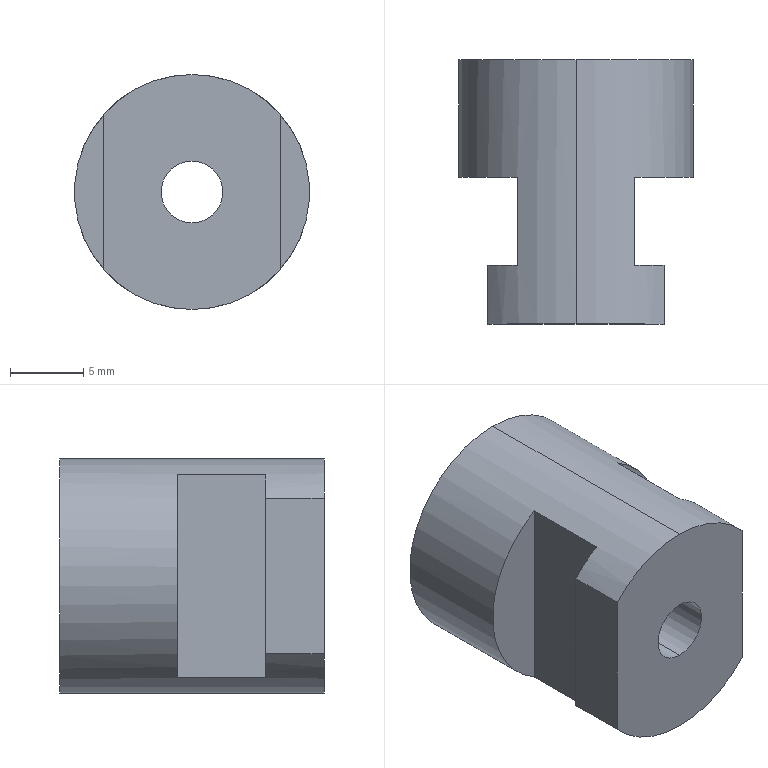Part | STEP file | 16 union cap | 1 solid | 14 faces | box 16 x 18 x 16 mm | volume 2782 mm3 | plane 10 | cylinder 4 | commonest cylinder face diameters 4.2 x2 16 x2
STEP:
#1=CARTESIAN_POINT('',(0.,0.,0.));
#2=DIRECTION('',(0.,0.,1.));
#3=DIRECTION('',(1.,0.,0.));
#4=AXIS2_PLACEMENT_3D('',#1,#2,#3);
#5=CARTESIAN_POINT('',(3.464,10.483,-2.1));
#6=VERTEX_POINT('',#5);
#7=CARTESIAN_POINT('',(3.464,-7.517,-2.1));
#8=VERTEX_POINT('',#7);
#9=CARTESIAN_POINT('',(3.464,-7.517,-2.1));
#10=DIRECTION('',(0.,-1.,0.));
#11=VECTOR('',#10,1.);
#12=LINE('',#9,#11);
#13=CARTESIAN_POINT('',(3.464,-7.517,0.));
#14=DIRECTION('',(0.,-1.,0.));
#15=DIRECTION('',(0.,0.,-1.));
#16=AXIS2_PLACEMENT_3D('',#13,#14,#15);
#17=CYLINDRICAL_SURFACE('',#16,2.1);
#18=CARTESIAN_POINT('',(6.283,0.));
#19=DIRECTION('',(0.,1.));
#20=VECTOR('',#19,1.);
#21=LINE('',#18,#20);
#22=(GEOMETRIC_REPRESENTATION_CONTEXT(2)PARAMETRIC_REPRESENTATION_CONTEXT()REPRESENTATION_CONTEXT('',''));
#23=DEFINITIONAL_REPRESENTATION('',(#21),#22);
#24=PCURVE('',#17,#23);
#25=CARTESIAN_POINT('',(3.464,-7.517,0.));
#26=DIRECTION('',(0.,-1.,0.));
#27=DIRECTION('',(0.,0.,-1.));
#28=AXIS2_PLACEMENT_3D('',#25,#26,#27);
#29=CYLINDRICAL_SURFACE('',#28,2.1);
#30=CARTESIAN_POINT('',(0.,0.));
#31=DIRECTION('',(0.,1.));
#32=VECTOR('',#31,1.);
#33=LINE('',#30,#32);
#34=(GEOMETRIC_REPRESENTATION_CONTEXT(2)PARAMETRIC_REPRESENTATION_CONTEXT()REPRESENTATION_CONTEXT('',''));
#35=DEFINITIONAL_REPRESENTATION('',(#33),#34);
#36=PCURVE('',#29,#35);
#37=SURFACE_CURVE('',#12,(#24,#36),.PCURVE_S1.);
#38=EDGE_CURVE('',#6,#8,#37,.T.);
#39=ORIENTED_EDGE('',*,*,#38,.T.);
#40=CARTESIAN_POINT('',(3.464,-7.517,2.1));
#41=VERTEX_POINT('',#40);
#42=CARTESIAN_POINT('',(3.464,-7.517,0.));
#43=DIRECTION('',(0.,-1.,0.));
#44=DIRECTION('',(0.,0.,-1.));
#45=AXIS2_PLACEMENT_3D('',#42,#43,#44);
#46=CIRCLE('',#45,2.1);
#47=CARTESIAN_POINT('',(0.,0.));
#48=DIRECTION('',(1.,0.));
#49=VECTOR('',#48,1.);
#50=LINE('',#47,#49);
#51=(GEOMETRIC_REPRESENTATION_CONTEXT(2)PARAMETRIC_REPRESENTATION_CONTEXT()REPRESENTATION_CONTEXT('',''));
#52=DEFINITIONAL_REPRESENTATION('',(#50),#51);
#53=PCURVE('',#17,#52);
#54=CARTESIAN_POINT('',(9.464,-7.517,-10.));
#55=DIRECTION('',(0.,-1.,0.));
#56=DIRECTION('',(0.,0.,-1.));
#57=AXIS2_PLACEMENT_3D('',#54,#55,#56);
#58=PLANE('',#57);
#59=CARTESIAN_POINT('',(-10.,-6.));
#60=DIRECTION('',(1.,0.));
#61=AXIS2_PLACEMENT_2D('',#59,#60);
#62=CIRCLE('',#61,2.1);
#63=(GEOMETRIC_REPRESENTATION_CONTEXT(2)PARAMETRIC_REPRESENTATION_CONTEXT()REPRESENTATION_CONTEXT('',''));
#64=DEFINITIONAL_REPRESENTATION('',(#62),#63);
#65=PCURVE('',#58,#64);
#66=SURFACE_CURVE('',#46,(#53,#65),.PCURVE_S1.);
#67=EDGE_CURVE('',#41,#8,#66,.T.);
#68=ORIENTED_EDGE('',*,*,#67,.F.);
#69=CARTESIAN_POINT('',(3.464,10.483,2.1));
#70=VERTEX_POINT('',#69);
#71=CARTESIAN_POINT('',(3.464,-7.517,2.1));
#72=DIRECTION('',(0.,-1.,0.));
#73=VECTOR('',#72,1.);
#74=LINE('',#71,#73);
#75=CARTESIAN_POINT('',(3.142,0.));
#76=DIRECTION('',(0.,1.));
#77=VECTOR('',#76,1.);
#78=LINE('',#75,#77);
#79=(GEOMETRIC_REPRESENTATION_CONTEXT(2)PARAMETRIC_REPRESENTATION_CONTEXT()REPRESENTATION_CONTEXT('',''));
#80=DEFINITIONAL_REPRESENTATION('',(#78),#79);
#81=PCURVE('',#17,#80);
#82=CARTESIAN_POINT('',(3.142,0.));
#83=DIRECTION('',(0.,1.));
#84=VECTOR('',#83,1.);
#85=LINE('',#82,#84);
#86=(GEOMETRIC_REPRESENTATION_CONTEXT(2)PARAMETRIC_REPRESENTATION_CONTEXT()REPRESENTATION_CONTEXT('',''));
#87=DEFINITIONAL_REPRESENTATION('',(#85),#86);
#88=PCURVE('',#29,#87);
#89=SURFACE_CURVE('',#74,(#81,#88),.PCURVE_S1.);
#90=EDGE_CURVE('',#70,#41,#89,.T.);
#91=ORIENTED_EDGE('',*,*,#90,.F.);
#92=CARTESIAN_POINT('',(3.464,10.483,0.));
#93=DIRECTION('',(0.,-1.,0.));
#94=DIRECTION('',(0.,0.,-1.));
#95=AXIS2_PLACEMENT_3D('',#92,#93,#94);
#96=CIRCLE('',#95,2.1);
#97=CARTESIAN_POINT('',(0.,-18.));
#98=DIRECTION('',(1.,0.));
#99=VECTOR('',#98,1.);
#100=LINE('',#97,#99);
#101=(GEOMETRIC_REPRESENTATION_CONTEXT(2)PARAMETRIC_REPRESENTATION_CONTEXT()REPRESENTATION_CONTEXT('',''));
#102=DEFINITIONAL_REPRESENTATION('',(#100),#101);
#103=PCURVE('',#17,#102);
#104=CARTESIAN_POINT('',(3.464,10.483,0.));
#105=DIRECTION('',(0.,1.,0.));
#106=DIRECTION('',(0.,0.,1.));
#107=AXIS2_PLACEMENT_3D('',#104,#105,#106);
#108=PLANE('',#107);
#109=CARTESIAN_POINT('',(-2.1,0.));
#110=CARTESIAN_POINT('',(-2.1,3.637));
#111=CARTESIAN_POINT('',(1.05,1.819));
#112=CARTESIAN_POINT('',(4.2,0.));
#113=CARTESIAN_POINT('',(1.05,-1.819));
#114=CARTESIAN_POINT('',(-2.1,-3.637));
#115=CARTESIAN_POINT('',(-2.1,0.));
#116=(BOUNDED_CURVE()B_SPLINE_CURVE(2,(#109,#110,#111,#112,#113,#114,#115),.UNSPECIFIED.,.T.,.F.)B_SPLINE_CURVE_WITH_KNOTS((1,2,2,2,2,1),(-2.094,0.,2.094,4.189,6.283,8.378),.UNSPECIFIED.)CURVE()GEOMETRIC_REPRESENTATION_ITEM()RATIONAL_B_SPLINE_CURVE((1.,0.5,1.,0.5,1.,0.5,1.))REPRESENTATION_ITEM(''));
#117=(GEOMETRIC_REPRESENTATION_CONTEXT(2)PARAMETRIC_REPRESENTATION_CONTEXT()REPRESENTATION_CONTEXT('',''));
#118=DEFINITIONAL_REPRESENTATION('',(#116),#117);
#119=PCURVE('',#108,#118);
#120=SURFACE_CURVE('',#96,(#103,#119),.PCURVE_S1.);
#121=EDGE_CURVE('',#70,#6,#120,.T.);
#122=ORIENTED_EDGE('',*,*,#121,.T.);
#123=EDGE_LOOP('',(#39,#68,#91,#122));
#124=FACE_BOUND('',#123,.F.);
#125=ADVANCED_FACE('',(#124),#17,.F.);
#126=CARTESIAN_POINT('',(9.464,-7.517,-5.292));
#127=VERTEX_POINT('',#126);
#128=CARTESIAN_POINT('',(3.464,-7.517,-8.));
#129=VERTEX_POINT('',#128);
#130=CARTESIAN_POINT('',(3.464,-7.517,0.));
#131=DIRECTION('',(0.,1.,0.));
#132=DIRECTION('',(0.,0.,1.));
#133=AXIS2_PLACEMENT_3D('',#130,#131,#132);
#134=CIRCLE('',#133,8.);
#135=CARTESIAN_POINT('',(3.464,-7.517,0.));
#136=DIRECTION('',(0.,1.,0.));
#137=DIRECTION('',(0.,0.,1.));
#138=AXIS2_PLACEMENT_3D('',#135,#136,#137);
#139=CYLINDRICAL_SURFACE('',#138,8.);
#140=CARTESIAN_POINT('',(0.,0.));
#141=DIRECTION('',(1.,0.));
#142=VECTOR('',#141,1.);
#143=LINE('',#140,#142);
#144=(GEOMETRIC_REPRESENTATION_CONTEXT(2)PARAMETRIC_REPRESENTATION_CONTEXT()REPRESENTATION_CONTEXT('',''));
#145=DEFINITIONAL_REPRESENTATION('',(#143),#144);
#146=PCURVE('',#139,#145);
#147=CARTESIAN_POINT('',(-18.,-6.));
#148=CARTESIAN_POINT('',(-18.,7.856));
#149=CARTESIAN_POINT('',(-6.,0.9282));
#150=CARTESIAN_POINT('',(6.,-6.));
#151=CARTESIAN_POINT('',(-6.,-12.928));
#152=CARTESIAN_POINT('',(-18.,-19.856));
#153=CARTESIAN_POINT('',(-18.,-6.));
#154=(BOUNDED_CURVE()B_SPLINE_CURVE(2,(#147,#148,#149,#150,#151,#152,#153),.UNSPECIFIED.,.T.,.F.)B_SPLINE_CURVE_WITH_KNOTS((1,2,2,2,2,1),(-2.094,0.,2.094,4.189,6.283,8.378),.UNSPECIFIED.)CURVE()GEOMETRIC_REPRESENTATION_ITEM()RATIONAL_B_SPLINE_CURVE((1.,0.5,1.,0.5,1.,0.5,1.))REPRESENTATION_ITEM(''));
#155=(GEOMETRIC_REPRESENTATION_CONTEXT(2)PARAMETRIC_REPRESENTATION_CONTEXT()REPRESENTATION_CONTEXT('',''));
#156=DEFINITIONAL_REPRESENTATION('',(#154),#155);
#157=PCURVE('',#58,#156);
#158=SURFACE_CURVE('',#134,(#146,#157),.PCURVE_S1.);
#159=EDGE_CURVE('',#127,#129,#158,.T.);
#160=ORIENTED_EDGE('',*,*,#159,.T.);
#161=CARTESIAN_POINT('',(3.464,10.483,-8.));
#162=VERTEX_POINT('',#161);
#163=CARTESIAN_POINT('',(3.464,-7.517,-8.));
#164=DIRECTION('',(0.,1.,0.));
#165=VECTOR('',#164,1.);
#166=LINE('',#163,#165);
#167=CARTESIAN_POINT('',(3.142,0.));
#168=DIRECTION('',(0.,1.));
#169=VECTOR('',#168,1.);
#170=LINE('',#167,#169);
#171=(GEOMETRIC_REPRESENTATION_CONTEXT(2)PARAMETRIC_REPRESENTATION_CONTEXT()REPRESENTATION_CONTEXT('',''));
#172=DEFINITIONAL_REPRESENTATION('',(#170),#171);
#173=PCURVE('',#139,#172);
#174=CARTESIAN_POINT('',(3.464,-7.517,0.));
#175=DIRECTION('',(0.,1.,0.));
#176=DIRECTION('',(0.,0.,1.));
#177=AXIS2_PLACEMENT_3D('',#174,#175,#176);
#178=CYLINDRICAL_SURFACE('',#177,8.);
#179=CARTESIAN_POINT('',(3.142,0.));
#180=DIRECTION('',(0.,1.));
#181=VECTOR('',#180,1.);
#182=LINE('',#179,#181);
#183=(GEOMETRIC_REPRESENTATION_CONTEXT(2)PARAMETRIC_REPRESENTATION_CONTEXT()REPRESENTATION_CONTEXT('',''));
#184=DEFINITIONAL_REPRESENTATION('',(#182),#183);
#185=PCURVE('',#178,#184);
#186=SURFACE_CURVE('',#166,(#173,#185),.PCURVE_S1.);
#187=EDGE_CURVE('',#129,#162,#186,.T.);
#188=ORIENTED_EDGE('',*,*,#187,.T.);
#189=CARTESIAN_POINT('',(3.464,10.483,8.));
#190=VERTEX_POINT('',#189);
#191=CARTESIAN_POINT('',(3.464,10.483,0.));
#192=DIRECTION('',(0.,1.,0.));
#193=DIRECTION('',(0.,0.,1.));
#194=AXIS2_PLACEMENT_3D('',#191,#192,#193);
#195=CIRCLE('',#194,8.);
#196=CARTESIAN_POINT('',(0.,18.));
#197=DIRECTION('',(1.,0.));
#198=VECTOR('',#197,1.);
#199=LINE('',#196,#198);
#200=(GEOMETRIC_REPRESENTATION_CONTEXT(2)PARAMETRIC_REPRESENTATION_CONTEXT()REPRESENTATION_CONTEXT('',''));
#201=DEFINITIONAL_REPRESENTATION('',(#199),#200);
#202=PCURVE('',#139,#201);
#203=CARTESIAN_POINT('',(0.,0.));
#204=DIRECTION('',(1.,0.));
#205=AXIS2_PLACEMENT_2D('',#203,#204);
#206=CIRCLE('',#205,8.);
#207=(GEOMETRIC_REPRESENTATION_CONTEXT(2)PARAMETRIC_REPRESENTATION_CONTEXT()REPRESENTATION_CONTEXT('',''));
#208=DEFINITIONAL_REPRESENTATION('',(#206),#207);
#209=PCURVE('',#108,#208);
#210=SURFACE_CURVE('',#195,(#202,#209),.PCURVE_S1.);
#211=EDGE_CURVE('',#190,#162,#210,.T.);
#212=ORIENTED_EDGE('',*,*,#211,.F.);
#213=CARTESIAN_POINT('',(3.464,-7.517,8.));
#214=VERTEX_POINT('',#213);
#215=CARTESIAN_POINT('',(3.464,-7.517,8.));
#216=DIRECTION('',(0.,1.,0.));
#217=VECTOR('',#216,1.);
#218=LINE('',#215,#217);
#219=CARTESIAN_POINT('',(0.,0.));
#220=DIRECTION('',(0.,1.));
#221=VECTOR('',#220,1.);
#222=LINE('',#219,#221);
#223=(GEOMETRIC_REPRESENTATION_CONTEXT(2)PARAMETRIC_REPRESENTATION_CONTEXT()REPRESENTATION_CONTEXT('',''));
#224=DEFINITIONAL_REPRESENTATION('',(#222),#223);
#225=PCURVE('',#139,#224);
#226=CARTESIAN_POINT('',(6.283,0.));
#227=DIRECTION('',(0.,1.));
#228=VECTOR('',#227,1.);
#229=LINE('',#226,#228);
#230=(GEOMETRIC_REPRESENTATION_CONTEXT(2)PARAMETRIC_REPRESENTATION_CONTEXT()REPRESENTATION_CONTEXT('',''));
#231=DEFINITIONAL_REPRESENTATION('',(#229),#230);
#232=PCURVE('',#178,#231);
#233=SURFACE_CURVE('',#218,(#225,#232),.PCURVE_S1.);
#234=EDGE_CURVE('',#214,#190,#233,.T.);
#235=ORIENTED_EDGE('',*,*,#234,.F.);
#236=CARTESIAN_POINT('',(9.464,-7.517,5.292));
#237=VERTEX_POINT('',#236);
#238=CARTESIAN_POINT('',(3.464,-7.517,0.));
#239=DIRECTION('',(0.,1.,0.));
#240=DIRECTION('',(0.,0.,1.));
#241=AXIS2_PLACEMENT_3D('',#238,#239,#240);
#242=CIRCLE('',#241,8.);
#243=CARTESIAN_POINT('',(0.,0.));
#244=DIRECTION('',(1.,0.));
#245=VECTOR('',#244,1.);
#246=LINE('',#243,#245);
#247=(GEOMETRIC_REPRESENTATION_CONTEXT(2)PARAMETRIC_REPRESENTATION_CONTEXT()REPRESENTATION_CONTEXT('',''));
#248=DEFINITIONAL_REPRESENTATION('',(#246),#247);
#249=PCURVE('',#139,#248);
#250=CARTESIAN_POINT('',(-18.,-6.));
#251=CARTESIAN_POINT('',(-18.,7.856));
#252=CARTESIAN_POINT('',(-6.,0.9282));
#253=CARTESIAN_POINT('',(6.,-6.));
#254=CARTESIAN_POINT('',(-6.,-12.928));
#255=CARTESIAN_POINT('',(-18.,-19.856));
#256=CARTESIAN_POINT('',(-18.,-6.));
#257=(BOUNDED_CURVE()B_SPLINE_CURVE(2,(#250,#251,#252,#253,#254,#255,#256),.UNSPECIFIED.,.T.,.F.)B_SPLINE_CURVE_WITH_KNOTS((1,2,2,2,2,1),(-2.094,0.,2.094,4.189,6.283,8.378),.UNSPECIFIED.)CURVE()GEOMETRIC_REPRESENTATION_ITEM()RATIONAL_B_SPLINE_CURVE((1.,0.5,1.,0.5,1.,0.5,1.))REPRESENTATION_ITEM(''));
#258=(GEOMETRIC_REPRESENTATION_CONTEXT(2)PARAMETRIC_REPRESENTATION_CONTEXT()REPRESENTATION_CONTEXT('',''));
#259=DEFINITIONAL_REPRESENTATION('',(#257),#258);
#260=PCURVE('',#58,#259);
#261=SURFACE_CURVE('',#242,(#249,#260),.PCURVE_S1.);
#262=EDGE_CURVE('',#214,#237,#261,.T.);
#263=ORIENTED_EDGE('',*,*,#262,.T.);
#264=CARTESIAN_POINT('',(9.464,-3.517,5.292));
#265=VERTEX_POINT('',#264);
#266=CARTESIAN_POINT('',(9.464,-7.517,5.292));
#267=DIRECTION('',(0.,-1.,0.));
#268=VECTOR('',#267,1.);
#269=LINE('',#266,#268);
#270=CARTESIAN_POINT('',(0.8481,0.));
#271=DIRECTION('',(0.,-1.));
#272=VECTOR('',#271,1.);
#273=LINE('',#270,#272);
#274=(GEOMETRIC_REPRESENTATION_CONTEXT(2)PARAMETRIC_REPRESENTATION_CONTEXT()REPRESENTATION_CONTEXT('',''));
#275=DEFINITIONAL_REPRESENTATION('',(#273),#274);
#276=PCURVE('',#139,#275);
#277=CARTESIAN_POINT('',(9.464,-7.517,-10.));
#278=DIRECTION('',(1.,0.,0.));
#279=DIRECTION('',(0.,0.,-1.));
#280=AXIS2_PLACEMENT_3D('',#277,#278,#279);
#281=PLANE('',#280);
#282=CARTESIAN_POINT('',(-15.292,0.));
#283=DIRECTION('',(0.,-1.));
#284=VECTOR('',#283,1.);
#285=LINE('',#282,#284);
#286=(GEOMETRIC_REPRESENTATION_CONTEXT(2)PARAMETRIC_REPRESENTATION_CONTEXT()REPRESENTATION_CONTEXT('',''));
#287=DEFINITIONAL_REPRESENTATION('',(#285),#286);
#288=PCURVE('',#281,#287);
#289=SURFACE_CURVE('',#269,(#276,#288),.PCURVE_S1.);
#290=EDGE_CURVE('',#265,#237,#289,.T.);
#291=ORIENTED_EDGE('',*,*,#290,.F.);
#292=CARTESIAN_POINT('',(7.464,-3.517,6.928));
#293=VERTEX_POINT('',#292);
#294=CARTESIAN_POINT('',(3.464,-3.517,0.));
#295=DIRECTION('',(0.,1.,0.));
#296=DIRECTION('',(-1.,0.,0.));
#297=AXIS2_PLACEMENT_3D('',#294,#295,#296);
#298=CIRCLE('',#297,8.);
#299=CARTESIAN_POINT('',(-1.571,4.));
#300=DIRECTION('',(1.,0.));
#301=VECTOR('',#300,1.);
#302=LINE('',#299,#301);
#303=(GEOMETRIC_REPRESENTATION_CONTEXT(2)PARAMETRIC_REPRESENTATION_CONTEXT()REPRESENTATION_CONTEXT('',''));
#304=DEFINITIONAL_REPRESENTATION('',(#302),#303);
#305=PCURVE('',#139,#304);
#306=CARTESIAN_POINT('',(9.464,-3.517,-10.));
#307=DIRECTION('',(0.,1.,0.));
#308=DIRECTION('',(-1.,0.,0.));
#309=AXIS2_PLACEMENT_3D('',#306,#307,#308);
#310=PLANE('',#309);
#311=CARTESIAN_POINT('',(6.,10.));
#312=DIRECTION('',(1.,0.));
#313=AXIS2_PLACEMENT_2D('',#311,#312);
#314=CIRCLE('',#313,8.);
#315=(GEOMETRIC_REPRESENTATION_CONTEXT(2)PARAMETRIC_REPRESENTATION_CONTEXT()REPRESENTATION_CONTEXT('',''));
#316=DEFINITIONAL_REPRESENTATION('',(#314),#315);
#317=PCURVE('',#310,#316);
#318=SURFACE_CURVE('',#298,(#305,#317),.PCURVE_S1.);
#319=EDGE_CURVE('',#293,#265,#318,.T.);
#320=ORIENTED_EDGE('',*,*,#319,.F.);
#321=CARTESIAN_POINT('',(7.464,2.483,6.928));
#322=VERTEX_POINT('',#321);
#323=CARTESIAN_POINT('',(7.464,-7.517,6.928));
#324=DIRECTION('',(0.,-1.,0.));
#325=VECTOR('',#324,1.);
#326=LINE('',#323,#325);
#327=CARTESIAN_POINT('',(0.5236,0.));
#328=DIRECTION('',(0.,-1.));
#329=VECTOR('',#328,1.);
#330=LINE('',#327,#329);
#331=(GEOMETRIC_REPRESENTATION_CONTEXT(2)PARAMETRIC_REPRESENTATION_CONTEXT()REPRESENTATION_CONTEXT('',''));
#332=DEFINITIONAL_REPRESENTATION('',(#330),#331);
#333=PCURVE('',#139,#332);
#334=CARTESIAN_POINT('',(7.464,-3.517,-10.));
#335=DIRECTION('',(1.,0.,0.));
#336=DIRECTION('',(0.,0.,-1.));
#337=AXIS2_PLACEMENT_3D('',#334,#335,#336);
#338=PLANE('',#337);
#339=CARTESIAN_POINT('',(-16.928,-4.));
#340=DIRECTION('',(0.,-1.));
#341=VECTOR('',#340,1.);
#342=LINE('',#339,#341);
#343=(GEOMETRIC_REPRESENTATION_CONTEXT(2)PARAMETRIC_REPRESENTATION_CONTEXT()REPRESENTATION_CONTEXT('',''));
#344=DEFINITIONAL_REPRESENTATION('',(#342),#343);
#345=PCURVE('',#338,#344);
#346=SURFACE_CURVE('',#326,(#333,#345),.PCURVE_S1.);
#347=EDGE_CURVE('',#322,#293,#346,.T.);
#348=ORIENTED_EDGE('',*,*,#347,.F.);
#349=CARTESIAN_POINT('',(7.464,2.483,-6.928));
#350=VERTEX_POINT('',#349);
#351=CARTESIAN_POINT('',(3.464,2.483,0.));
#352=DIRECTION('',(0.,1.,0.));
#353=DIRECTION('',(0.,0.,1.));
#354=AXIS2_PLACEMENT_3D('',#351,#352,#353);
#355=CIRCLE('',#354,8.);
#356=CARTESIAN_POINT('',(0.,10.));
#357=DIRECTION('',(1.,0.));
#358=VECTOR('',#357,1.);
#359=LINE('',#356,#358);
#360=(GEOMETRIC_REPRESENTATION_CONTEXT(2)PARAMETRIC_REPRESENTATION_CONTEXT()REPRESENTATION_CONTEXT('',''));
#361=DEFINITIONAL_REPRESENTATION('',(#359),#360);
#362=PCURVE('',#139,#361);
#363=CARTESIAN_POINT('',(3.464,2.483,0.));
#364=DIRECTION('',(0.,1.,0.));
#365=DIRECTION('',(0.,0.,1.));
#366=AXIS2_PLACEMENT_3D('',#363,#364,#365);
#367=PLANE('',#366);
#368=CARTESIAN_POINT('',(0.,0.));
#369=DIRECTION('',(1.,0.));
#370=AXIS2_PLACEMENT_2D('',#368,#369);
#371=CIRCLE('',#370,8.);
#372=(GEOMETRIC_REPRESENTATION_CONTEXT(2)PARAMETRIC_REPRESENTATION_CONTEXT()REPRESENTATION_CONTEXT('',''));
#373=DEFINITIONAL_REPRESENTATION('',(#371),#372);
#374=PCURVE('',#367,#373);
#375=SURFACE_CURVE('',#355,(#362,#374),.PCURVE_S1.);
#376=EDGE_CURVE('',#322,#350,#375,.T.);
#377=ORIENTED_EDGE('',*,*,#376,.T.);
#378=CARTESIAN_POINT('',(7.464,-3.517,-6.928));
#379=VERTEX_POINT('',#378);
#380=CARTESIAN_POINT('',(7.464,-7.517,-6.928));
#381=DIRECTION('',(0.,1.,0.));
#382=VECTOR('',#381,1.);
#383=LINE('',#380,#382);
#384=CARTESIAN_POINT('',(2.618,0.));
#385=DIRECTION('',(0.,1.));
#386=VECTOR('',#385,1.);
#387=LINE('',#384,#386);
#388=(GEOMETRIC_REPRESENTATION_CONTEXT(2)PARAMETRIC_REPRESENTATION_CONTEXT()REPRESENTATION_CONTEXT('',''));
#389=DEFINITIONAL_REPRESENTATION('',(#387),#388);
#390=PCURVE('',#139,#389);
#391=CARTESIAN_POINT('',(-3.072,-4.));
#392=DIRECTION('',(0.,1.));
#393=VECTOR('',#392,1.);
#394=LINE('',#391,#393);
#395=(GEOMETRIC_REPRESENTATION_CONTEXT(2)PARAMETRIC_REPRESENTATION_CONTEXT()REPRESENTATION_CONTEXT('',''));
#396=DEFINITIONAL_REPRESENTATION('',(#394),#395);
#397=PCURVE('',#338,#396);
#398=SURFACE_CURVE('',#383,(#390,#397),.PCURVE_S1.);
#399=EDGE_CURVE('',#379,#350,#398,.T.);
#400=ORIENTED_EDGE('',*,*,#399,.F.);
#401=CARTESIAN_POINT('',(9.464,-3.517,-5.292));
#402=VERTEX_POINT('',#401);
#403=CARTESIAN_POINT('',(3.464,-3.517,0.));
#404=DIRECTION('',(0.,1.,0.));
#405=DIRECTION('',(-1.,0.,0.));
#406=AXIS2_PLACEMENT_3D('',#403,#404,#405);
#407=CIRCLE('',#406,8.);
#408=CARTESIAN_POINT('',(-1.571,4.));
#409=DIRECTION('',(1.,0.));
#410=VECTOR('',#409,1.);
#411=LINE('',#408,#410);
#412=(GEOMETRIC_REPRESENTATION_CONTEXT(2)PARAMETRIC_REPRESENTATION_CONTEXT()REPRESENTATION_CONTEXT('',''));
#413=DEFINITIONAL_REPRESENTATION('',(#411),#412);
#414=PCURVE('',#139,#413);
#415=CARTESIAN_POINT('',(6.,10.));
#416=DIRECTION('',(1.,0.));
#417=AXIS2_PLACEMENT_2D('',#415,#416);
#418=CIRCLE('',#417,8.);
#419=(GEOMETRIC_REPRESENTATION_CONTEXT(2)PARAMETRIC_REPRESENTATION_CONTEXT()REPRESENTATION_CONTEXT('',''));
#420=DEFINITIONAL_REPRESENTATION('',(#418),#419);
#421=PCURVE('',#310,#420);
#422=SURFACE_CURVE('',#407,(#414,#421),.PCURVE_S1.);
#423=EDGE_CURVE('',#402,#379,#422,.T.);
#424=ORIENTED_EDGE('',*,*,#423,.F.);
#425=CARTESIAN_POINT('',(9.464,-7.517,-5.292));
#426=DIRECTION('',(0.,1.,0.));
#427=VECTOR('',#426,1.);
#428=LINE('',#425,#427);
#429=CARTESIAN_POINT('',(2.294,0.));
#430=DIRECTION('',(0.,1.));
#431=VECTOR('',#430,1.);
#432=LINE('',#429,#431);
#433=(GEOMETRIC_REPRESENTATION_CONTEXT(2)PARAMETRIC_REPRESENTATION_CONTEXT()REPRESENTATION_CONTEXT('',''));
#434=DEFINITIONAL_REPRESENTATION('',(#432),#433);
#435=PCURVE('',#139,#434);
#436=CARTESIAN_POINT('',(-4.708,0.));
#437=DIRECTION('',(0.,1.));
#438=VECTOR('',#437,1.);
#439=LINE('',#436,#438);
#440=(GEOMETRIC_REPRESENTATION_CONTEXT(2)PARAMETRIC_REPRESENTATION_CONTEXT()REPRESENTATION_CONTEXT('',''));
#441=DEFINITIONAL_REPRESENTATION('',(#439),#440);
#442=PCURVE('',#281,#441);
#443=SURFACE_CURVE('',#428,(#435,#442),.PCURVE_S1.);
#444=EDGE_CURVE('',#127,#402,#443,.T.);
#445=ORIENTED_EDGE('',*,*,#444,.F.);
#446=EDGE_LOOP('',(#160,#188,#212,#235,#263,#291,#320,#348,#377,#400,#424,#445));
#447=FACE_BOUND('',#446,.T.);
#448=ADVANCED_FACE('',(#447),#139,.T.);
#449=CARTESIAN_POINT('',(7.464,-3.517,-10.));
#450=DIRECTION('',(0.,0.,1.));
#451=VECTOR('',#450,1.);
#452=LINE('',#449,#451);
#453=CARTESIAN_POINT('',(2.,0.));
#454=DIRECTION('',(0.,1.));
#455=VECTOR('',#454,1.);
#456=LINE('',#453,#455);
#457=(GEOMETRIC_REPRESENTATION_CONTEXT(2)PARAMETRIC_REPRESENTATION_CONTEXT()REPRESENTATION_CONTEXT('',''));
#458=DEFINITIONAL_REPRESENTATION('',(#456),#457);
#459=PCURVE('',#310,#458);
#460=CARTESIAN_POINT('',(0.,0.));
#461=DIRECTION('',(-1.,0.));
#462=VECTOR('',#461,1.);
#463=LINE('',#460,#462);
#464=(GEOMETRIC_REPRESENTATION_CONTEXT(2)PARAMETRIC_REPRESENTATION_CONTEXT()REPRESENTATION_CONTEXT('',''));
#465=DEFINITIONAL_REPRESENTATION('',(#463),#464);
#466=PCURVE('',#338,#465);
#467=SURFACE_CURVE('',#452,(#459,#466),.PCURVE_S1.);
#468=EDGE_CURVE('',#379,#293,#467,.T.);
#469=ORIENTED_EDGE('',*,*,#468,.T.);
#470=ORIENTED_EDGE('',*,*,#319,.T.);
#471=CARTESIAN_POINT('',(9.464,-3.517,-10.));
#472=DIRECTION('',(0.,0.,1.));
#473=VECTOR('',#472,1.);
#474=LINE('',#471,#473);
#475=CARTESIAN_POINT('',(0.,0.));
#476=DIRECTION('',(0.,1.));
#477=VECTOR('',#476,1.);
#478=LINE('',#475,#477);
#479=(GEOMETRIC_REPRESENTATION_CONTEXT(2)PARAMETRIC_REPRESENTATION_CONTEXT()REPRESENTATION_CONTEXT('',''));
#480=DEFINITIONAL_REPRESENTATION('',(#478),#479);
#481=PCURVE('',#310,#480);
#482=CARTESIAN_POINT('',(0.,4.));
#483=DIRECTION('',(-1.,0.));
#484=VECTOR('',#483,1.);
#485=LINE('',#482,#484);
#486=(GEOMETRIC_REPRESENTATION_CONTEXT(2)PARAMETRIC_REPRESENTATION_CONTEXT()REPRESENTATION_CONTEXT('',''));
#487=DEFINITIONAL_REPRESENTATION('',(#485),#486);
#488=PCURVE('',#281,#487);
#489=SURFACE_CURVE('',#474,(#481,#488),.PCURVE_S1.);
#490=EDGE_CURVE('',#402,#265,#489,.T.);
#491=ORIENTED_EDGE('',*,*,#490,.F.);
#492=ORIENTED_EDGE('',*,*,#423,.T.);
#493=EDGE_LOOP('',(#469,#470,#491,#492));
#494=FACE_BOUND('',#493,.T.);
#495=ADVANCED_FACE('',(#494),#310,.T.);
#496=CARTESIAN_POINT('',(9.464,-7.517,-10.));
#497=DIRECTION('',(0.,0.,1.));
#498=VECTOR('',#497,1.);
#499=LINE('',#496,#498);
#500=CARTESIAN_POINT('',(0.,0.));
#501=DIRECTION('',(-1.,0.));
#502=VECTOR('',#501,1.);
#503=LINE('',#500,#502);
#504=(GEOMETRIC_REPRESENTATION_CONTEXT(2)PARAMETRIC_REPRESENTATION_CONTEXT()REPRESENTATION_CONTEXT('',''));
#505=DEFINITIONAL_REPRESENTATION('',(#503),#504);
#506=PCURVE('',#281,#505);
#507=CARTESIAN_POINT('',(0.,0.));
#508=DIRECTION('',(-1.,0.));
#509=VECTOR('',#508,1.);
#510=LINE('',#507,#509);
#511=(GEOMETRIC_REPRESENTATION_CONTEXT(2)PARAMETRIC_REPRESENTATION_CONTEXT()REPRESENTATION_CONTEXT('',''));
#512=DEFINITIONAL_REPRESENTATION('',(#510),#511);
#513=PCURVE('',#58,#512);
#514=SURFACE_CURVE('',#499,(#506,#513),.PCURVE_S1.);
#515=EDGE_CURVE('',#127,#237,#514,.T.);
#516=ORIENTED_EDGE('',*,*,#515,.F.);
#517=ORIENTED_EDGE('',*,*,#444,.T.);
#518=ORIENTED_EDGE('',*,*,#490,.T.);
#519=ORIENTED_EDGE('',*,*,#290,.T.);
#520=EDGE_LOOP('',(#516,#517,#518,#519));
#521=FACE_BOUND('',#520,.T.);
#522=ADVANCED_FACE('',(#521),#281,.T.);
#523=CARTESIAN_POINT('',(3.464,-7.517,0.));
#524=DIRECTION('',(0.,-1.,0.));
#525=DIRECTION('',(0.,0.,-1.));
#526=AXIS2_PLACEMENT_3D('',#523,#524,#525);
#527=CIRCLE('',#526,2.1);
#528=CARTESIAN_POINT('',(-10.,-6.));
#529=DIRECTION('',(1.,0.));
#530=AXIS2_PLACEMENT_2D('',#528,#529);
#531=CIRCLE('',#530,2.1);
#532=(GEOMETRIC_REPRESENTATION_CONTEXT(2)PARAMETRIC_REPRESENTATION_CONTEXT()REPRESENTATION_CONTEXT('',''));
#533=DEFINITIONAL_REPRESENTATION('',(#531),#532);
#534=PCURVE('',#58,#533);
#535=CARTESIAN_POINT('',(0.,0.));
#536=DIRECTION('',(1.,0.));
#537=VECTOR('',#536,1.);
#538=LINE('',#535,#537);
#539=(GEOMETRIC_REPRESENTATION_CONTEXT(2)PARAMETRIC_REPRESENTATION_CONTEXT()REPRESENTATION_CONTEXT('',''));
#540=DEFINITIONAL_REPRESENTATION('',(#538),#539);
#541=PCURVE('',#29,#540);
#542=SURFACE_CURVE('',#527,(#534,#541),.PCURVE_S1.);
#543=EDGE_CURVE('',#8,#41,#542,.T.);
#544=ORIENTED_EDGE('',*,*,#543,.F.);
#545=ORIENTED_EDGE('',*,*,#67,.F.);
#546=EDGE_LOOP('',(#544,#545));
#547=FACE_BOUND('',#546,.T.);
#548=ORIENTED_EDGE('',*,*,#515,.T.);
#549=ORIENTED_EDGE('',*,*,#262,.F.);
#550=CARTESIAN_POINT('',(-2.536,-7.517,5.292));
#551=VERTEX_POINT('',#550);
#552=CARTESIAN_POINT('',(3.464,-7.517,0.));
#553=DIRECTION('',(0.,1.,0.));
#554=DIRECTION('',(0.,0.,1.));
#555=AXIS2_PLACEMENT_3D('',#552,#553,#554);
#556=CIRCLE('',#555,8.);
#557=CARTESIAN_POINT('',(-18.,-6.));
#558=CARTESIAN_POINT('',(-18.,7.856));
#559=CARTESIAN_POINT('',(-6.,0.9282));
#560=CARTESIAN_POINT('',(6.,-6.));
#561=CARTESIAN_POINT('',(-6.,-12.928));
#562=CARTESIAN_POINT('',(-18.,-19.856));
#563=CARTESIAN_POINT('',(-18.,-6.));
#564=(BOUNDED_CURVE()B_SPLINE_CURVE(2,(#557,#558,#559,#560,#561,#562,#563),.UNSPECIFIED.,.T.,.F.)B_SPLINE_CURVE_WITH_KNOTS((1,2,2,2,2,1),(-2.094,0.,2.094,4.189,6.283,8.378),.UNSPECIFIED.)CURVE()GEOMETRIC_REPRESENTATION_ITEM()RATIONAL_B_SPLINE_CURVE((1.,0.5,1.,0.5,1.,0.5,1.))REPRESENTATION_ITEM(''));
#565=(GEOMETRIC_REPRESENTATION_CONTEXT(2)PARAMETRIC_REPRESENTATION_CONTEXT()REPRESENTATION_CONTEXT('',''));
#566=DEFINITIONAL_REPRESENTATION('',(#564),#565);
#567=PCURVE('',#58,#566);
#568=CARTESIAN_POINT('',(0.,0.));
#569=DIRECTION('',(1.,0.));
#570=VECTOR('',#569,1.);
#571=LINE('',#568,#570);
#572=(GEOMETRIC_REPRESENTATION_CONTEXT(2)PARAMETRIC_REPRESENTATION_CONTEXT()REPRESENTATION_CONTEXT('',''));
#573=DEFINITIONAL_REPRESENTATION('',(#571),#572);
#574=PCURVE('',#178,#573);
#575=SURFACE_CURVE('',#556,(#567,#574),.PCURVE_S1.);
#576=EDGE_CURVE('',#551,#214,#575,.T.);
#577=ORIENTED_EDGE('',*,*,#576,.F.);
#578=CARTESIAN_POINT('',(-2.536,-7.517,-5.292));
#579=VERTEX_POINT('',#578);
#580=CARTESIAN_POINT('',(-2.536,-7.517,-10.));
#581=DIRECTION('',(0.,0.,1.));
#582=VECTOR('',#581,1.);
#583=LINE('',#580,#582);
#584=CARTESIAN_POINT('',(0.,-12.));
#585=DIRECTION('',(-1.,0.));
#586=VECTOR('',#585,1.);
#587=LINE('',#584,#586);
#588=(GEOMETRIC_REPRESENTATION_CONTEXT(2)PARAMETRIC_REPRESENTATION_CONTEXT()REPRESENTATION_CONTEXT('',''));
#589=DEFINITIONAL_REPRESENTATION('',(#587),#588);
#590=PCURVE('',#58,#589);
#591=CARTESIAN_POINT('',(-2.536,-7.517,-10.));
#592=DIRECTION('',(-1.,0.,0.));
#593=DIRECTION('',(0.,0.,1.));
#594=AXIS2_PLACEMENT_3D('',#591,#592,#593);
#595=PLANE('',#594);
#596=CARTESIAN_POINT('',(0.,0.));
#597=DIRECTION('',(1.,0.));
#598=VECTOR('',#597,1.);
#599=LINE('',#596,#598);
#600=(GEOMETRIC_REPRESENTATION_CONTEXT(2)PARAMETRIC_REPRESENTATION_CONTEXT()REPRESENTATION_CONTEXT('',''));
#601=DEFINITIONAL_REPRESENTATION('',(#599),#600);
#602=PCURVE('',#595,#601);
#603=SURFACE_CURVE('',#583,(#590,#602),.PCURVE_S1.);
#604=EDGE_CURVE('',#579,#551,#603,.T.);
#605=ORIENTED_EDGE('',*,*,#604,.F.);
#606=CARTESIAN_POINT('',(3.464,-7.517,0.));
#607=DIRECTION('',(0.,1.,0.));
#608=DIRECTION('',(0.,0.,1.));
#609=AXIS2_PLACEMENT_3D('',#606,#607,#608);
#610=CIRCLE('',#609,8.);
#611=CARTESIAN_POINT('',(-18.,-6.));
#612=CARTESIAN_POINT('',(-18.,7.856));
#613=CARTESIAN_POINT('',(-6.,0.9282));
#614=CARTESIAN_POINT('',(6.,-6.));
#615=CARTESIAN_POINT('',(-6.,-12.928));
#616=CARTESIAN_POINT('',(-18.,-19.856));
#617=CARTESIAN_POINT('',(-18.,-6.));
#618=(BOUNDED_CURVE()B_SPLINE_CURVE(2,(#611,#612,#613,#614,#615,#616,#617),.UNSPECIFIED.,.T.,.F.)B_SPLINE_CURVE_WITH_KNOTS((1,2,2,2,2,1),(-2.094,0.,2.094,4.189,6.283,8.378),.UNSPECIFIED.)CURVE()GEOMETRIC_REPRESENTATION_ITEM()RATIONAL_B_SPLINE_CURVE((1.,0.5,1.,0.5,1.,0.5,1.))REPRESENTATION_ITEM(''));
#619=(GEOMETRIC_REPRESENTATION_CONTEXT(2)PARAMETRIC_REPRESENTATION_CONTEXT()REPRESENTATION_CONTEXT('',''));
#620=DEFINITIONAL_REPRESENTATION('',(#618),#619);
#621=PCURVE('',#58,#620);
#622=CARTESIAN_POINT('',(0.,0.));
#623=DIRECTION('',(1.,0.));
#624=VECTOR('',#623,1.);
#625=LINE('',#622,#624);
#626=(GEOMETRIC_REPRESENTATION_CONTEXT(2)PARAMETRIC_REPRESENTATION_CONTEXT()REPRESENTATION_CONTEXT('',''));
#627=DEFINITIONAL_REPRESENTATION('',(#625),#626);
#628=PCURVE('',#178,#627);
#629=SURFACE_CURVE('',#610,(#621,#628),.PCURVE_S1.);
#630=EDGE_CURVE('',#129,#579,#629,.T.);
#631=ORIENTED_EDGE('',*,*,#630,.F.);
#632=ORIENTED_EDGE('',*,*,#159,.F.);
#633=EDGE_LOOP('',(#548,#549,#577,#605,#631,#632));
#634=FACE_BOUND('',#633,.T.);
#635=ADVANCED_FACE('',(#547,#634),#58,.T.);
#636=ORIENTED_EDGE('',*,*,#604,.T.);
#637=CARTESIAN_POINT('',(-2.536,-3.517,5.292));
#638=VERTEX_POINT('',#637);
#639=CARTESIAN_POINT('',(-2.536,-7.517,5.292));
#640=DIRECTION('',(0.,1.,0.));
#641=VECTOR('',#640,1.);
#642=LINE('',#639,#641);
#643=CARTESIAN_POINT('',(15.292,0.));
#644=DIRECTION('',(0.,1.));
#645=VECTOR('',#644,1.);
#646=LINE('',#643,#645);
#647=(GEOMETRIC_REPRESENTATION_CONTEXT(2)PARAMETRIC_REPRESENTATION_CONTEXT()REPRESENTATION_CONTEXT('',''));
#648=DEFINITIONAL_REPRESENTATION('',(#646),#647);
#649=PCURVE('',#595,#648);
#650=CARTESIAN_POINT('',(5.435,0.));
#651=DIRECTION('',(0.,1.));
#652=VECTOR('',#651,1.);
#653=LINE('',#650,#652);
#654=(GEOMETRIC_REPRESENTATION_CONTEXT(2)PARAMETRIC_REPRESENTATION_CONTEXT()REPRESENTATION_CONTEXT('',''));
#655=DEFINITIONAL_REPRESENTATION('',(#653),#654);
#656=PCURVE('',#178,#655);
#657=SURFACE_CURVE('',#642,(#649,#656),.PCURVE_S1.);
#658=EDGE_CURVE('',#551,#638,#657,.T.);
#659=ORIENTED_EDGE('',*,*,#658,.T.);
#660=CARTESIAN_POINT('',(-2.536,-3.517,-5.292));
#661=VERTEX_POINT('',#660);
#662=CARTESIAN_POINT('',(-2.536,-3.517,-10.));
#663=DIRECTION('',(0.,0.,1.));
#664=VECTOR('',#663,1.);
#665=LINE('',#662,#664);
#666=CARTESIAN_POINT('',(0.,4.));
#667=DIRECTION('',(1.,0.));
#668=VECTOR('',#667,1.);
#669=LINE('',#666,#668);
#670=(GEOMETRIC_REPRESENTATION_CONTEXT(2)PARAMETRIC_REPRESENTATION_CONTEXT()REPRESENTATION_CONTEXT('',''));
#671=DEFINITIONAL_REPRESENTATION('',(#669),#670);
#672=PCURVE('',#595,#671);
#673=CARTESIAN_POINT('',(-2.536,-3.517,-10.));
#674=DIRECTION('',(0.,1.,0.));
#675=DIRECTION('',(-1.,0.,0.));
#676=AXIS2_PLACEMENT_3D('',#673,#674,#675);
#677=PLANE('',#676);
#678=CARTESIAN_POINT('',(0.,0.));
#679=DIRECTION('',(0.,1.));
#680=VECTOR('',#679,1.);
#681=LINE('',#678,#680);
#682=(GEOMETRIC_REPRESENTATION_CONTEXT(2)PARAMETRIC_REPRESENTATION_CONTEXT()REPRESENTATION_CONTEXT('',''));
#683=DEFINITIONAL_REPRESENTATION('',(#681),#682);
#684=PCURVE('',#677,#683);
#685=SURFACE_CURVE('',#665,(#672,#684),.PCURVE_S1.);
#686=EDGE_CURVE('',#661,#638,#685,.T.);
#687=ORIENTED_EDGE('',*,*,#686,.F.);
#688=CARTESIAN_POINT('',(-2.536,-7.517,-5.292));
#689=DIRECTION('',(0.,-1.,0.));
#690=VECTOR('',#689,1.);
#691=LINE('',#688,#690);
#692=CARTESIAN_POINT('',(4.708,0.));
#693=DIRECTION('',(0.,-1.));
#694=VECTOR('',#693,1.);
#695=LINE('',#692,#694);
#696=(GEOMETRIC_REPRESENTATION_CONTEXT(2)PARAMETRIC_REPRESENTATION_CONTEXT()REPRESENTATION_CONTEXT('',''));
#697=DEFINITIONAL_REPRESENTATION('',(#695),#696);
#698=PCURVE('',#595,#697);
#699=CARTESIAN_POINT('',(3.99,0.));
#700=DIRECTION('',(0.,-1.));
#701=VECTOR('',#700,1.);
#702=LINE('',#699,#701);
#703=(GEOMETRIC_REPRESENTATION_CONTEXT(2)PARAMETRIC_REPRESENTATION_CONTEXT()REPRESENTATION_CONTEXT('',''));
#704=DEFINITIONAL_REPRESENTATION('',(#702),#703);
#705=PCURVE('',#178,#704);
#706=SURFACE_CURVE('',#691,(#698,#705),.PCURVE_S1.);
#707=EDGE_CURVE('',#661,#579,#706,.T.);
#708=ORIENTED_EDGE('',*,*,#707,.T.);
#709=EDGE_LOOP('',(#636,#659,#687,#708));
#710=FACE_BOUND('',#709,.T.);
#711=ADVANCED_FACE('',(#710),#595,.T.);
#712=ORIENTED_EDGE('',*,*,#686,.T.);
#713=CARTESIAN_POINT('',(-0.5357,-3.517,6.928));
#714=VERTEX_POINT('',#713);
#715=CARTESIAN_POINT('',(3.464,-3.517,0.));
#716=DIRECTION('',(0.,1.,0.));
#717=DIRECTION('',(-1.,0.,0.));
#718=AXIS2_PLACEMENT_3D('',#715,#716,#717);
#719=CIRCLE('',#718,8.);
#720=CARTESIAN_POINT('',(-6.,10.));
#721=DIRECTION('',(1.,0.));
#722=AXIS2_PLACEMENT_2D('',#720,#721);
#723=CIRCLE('',#722,8.);
#724=(GEOMETRIC_REPRESENTATION_CONTEXT(2)PARAMETRIC_REPRESENTATION_CONTEXT()REPRESENTATION_CONTEXT('',''));
#725=DEFINITIONAL_REPRESENTATION('',(#723),#724);
#726=PCURVE('',#677,#725);
#727=CARTESIAN_POINT('',(4.712,4.));
#728=DIRECTION('',(1.,0.));
#729=VECTOR('',#728,1.);
#730=LINE('',#727,#729);
#731=(GEOMETRIC_REPRESENTATION_CONTEXT(2)PARAMETRIC_REPRESENTATION_CONTEXT()REPRESENTATION_CONTEXT('',''));
#732=DEFINITIONAL_REPRESENTATION('',(#730),#731);
#733=PCURVE('',#178,#732);
#734=SURFACE_CURVE('',#719,(#726,#733),.PCURVE_S1.);
#735=EDGE_CURVE('',#638,#714,#734,.T.);
#736=ORIENTED_EDGE('',*,*,#735,.T.);
#737=CARTESIAN_POINT('',(-0.5357,-3.517,-6.928));
#738=VERTEX_POINT('',#737);
#739=CARTESIAN_POINT('',(-0.5357,-3.517,-10.));
#740=DIRECTION('',(0.,0.,1.));
#741=VECTOR('',#740,1.);
#742=LINE('',#739,#741);
#743=CARTESIAN_POINT('',(-2.,0.));
#744=DIRECTION('',(0.,1.));
#745=VECTOR('',#744,1.);
#746=LINE('',#743,#745);
#747=(GEOMETRIC_REPRESENTATION_CONTEXT(2)PARAMETRIC_REPRESENTATION_CONTEXT()REPRESENTATION_CONTEXT('',''));
#748=DEFINITIONAL_REPRESENTATION('',(#746),#747);
#749=PCURVE('',#677,#748);
#750=CARTESIAN_POINT('',(-0.5357,-3.517,-10.));
#751=DIRECTION('',(-1.,0.,0.));
#752=DIRECTION('',(0.,0.,1.));
#753=AXIS2_PLACEMENT_3D('',#750,#751,#752);
#754=PLANE('',#753);
#755=CARTESIAN_POINT('',(0.,0.));
#756=DIRECTION('',(1.,0.));
#757=VECTOR('',#756,1.);
#758=LINE('',#755,#757);
#759=(GEOMETRIC_REPRESENTATION_CONTEXT(2)PARAMETRIC_REPRESENTATION_CONTEXT()REPRESENTATION_CONTEXT('',''));
#760=DEFINITIONAL_REPRESENTATION('',(#758),#759);
#761=PCURVE('',#754,#760);
#762=SURFACE_CURVE('',#742,(#749,#761),.PCURVE_S1.);
#763=EDGE_CURVE('',#738,#714,#762,.T.);
#764=ORIENTED_EDGE('',*,*,#763,.F.);
#765=CARTESIAN_POINT('',(3.464,-3.517,0.));
#766=DIRECTION('',(0.,1.,0.));
#767=DIRECTION('',(-1.,0.,0.));
#768=AXIS2_PLACEMENT_3D('',#765,#766,#767);
#769=CIRCLE('',#768,8.);
#770=CARTESIAN_POINT('',(-6.,10.));
#771=DIRECTION('',(1.,0.));
#772=AXIS2_PLACEMENT_2D('',#770,#771);
#773=CIRCLE('',#772,8.);
#774=(GEOMETRIC_REPRESENTATION_CONTEXT(2)PARAMETRIC_REPRESENTATION_CONTEXT()REPRESENTATION_CONTEXT('',''));
#775=DEFINITIONAL_REPRESENTATION('',(#773),#774);
#776=PCURVE('',#677,#775);
#777=CARTESIAN_POINT('',(-1.571,4.));
#778=DIRECTION('',(1.,0.));
#779=VECTOR('',#778,1.);
#780=LINE('',#777,#779);
#781=(GEOMETRIC_REPRESENTATION_CONTEXT(2)PARAMETRIC_REPRESENTATION_CONTEXT()REPRESENTATION_CONTEXT('',''));
#782=DEFINITIONAL_REPRESENTATION('',(#780),#781);
#783=PCURVE('',#178,#782);
#784=SURFACE_CURVE('',#769,(#776,#783),.PCURVE_S1.);
#785=EDGE_CURVE('',#738,#661,#784,.T.);
#786=ORIENTED_EDGE('',*,*,#785,.T.);
#787=EDGE_LOOP('',(#712,#736,#764,#786));
#788=FACE_BOUND('',#787,.T.);
#789=ADVANCED_FACE('',(#788),#677,.T.);
#790=ORIENTED_EDGE('',*,*,#763,.T.);
#791=CARTESIAN_POINT('',(-0.5357,2.483,6.928));
#792=VERTEX_POINT('',#791);
#793=CARTESIAN_POINT('',(-0.5357,-7.517,6.928));
#794=DIRECTION('',(0.,1.,0.));
#795=VECTOR('',#794,1.);
#796=LINE('',#793,#795);
#797=CARTESIAN_POINT('',(16.928,-4.));
#798=DIRECTION('',(0.,1.));
#799=VECTOR('',#798,1.);
#800=LINE('',#797,#799);
#801=(GEOMETRIC_REPRESENTATION_CONTEXT(2)PARAMETRIC_REPRESENTATION_CONTEXT()REPRESENTATION_CONTEXT('',''));
#802=DEFINITIONAL_REPRESENTATION('',(#800),#801);
#803=PCURVE('',#754,#802);
#804=CARTESIAN_POINT('',(5.76,0.));
#805=DIRECTION('',(0.,1.));
#806=VECTOR('',#805,1.);
#807=LINE('',#804,#806);
#808=(GEOMETRIC_REPRESENTATION_CONTEXT(2)PARAMETRIC_REPRESENTATION_CONTEXT()REPRESENTATION_CONTEXT('',''));
#809=DEFINITIONAL_REPRESENTATION('',(#807),#808);
#810=PCURVE('',#178,#809);
#811=SURFACE_CURVE('',#796,(#803,#810),.PCURVE_S1.);
#812=EDGE_CURVE('',#714,#792,#811,.T.);
#813=ORIENTED_EDGE('',*,*,#812,.T.);
#814=CARTESIAN_POINT('',(-0.5357,2.483,-6.928));
#815=VERTEX_POINT('',#814);
#816=CARTESIAN_POINT('',(-0.5357,2.483,-10.));
#817=DIRECTION('',(0.,0.,1.));
#818=VECTOR('',#817,1.);
#819=LINE('',#816,#818);
#820=CARTESIAN_POINT('',(0.,6.));
#821=DIRECTION('',(1.,0.));
#822=VECTOR('',#821,1.);
#823=LINE('',#820,#822);
#824=(GEOMETRIC_REPRESENTATION_CONTEXT(2)PARAMETRIC_REPRESENTATION_CONTEXT()REPRESENTATION_CONTEXT('',''));
#825=DEFINITIONAL_REPRESENTATION('',(#823),#824);
#826=PCURVE('',#754,#825);
#827=CARTESIAN_POINT('',(3.464,2.483,0.));
#828=DIRECTION('',(0.,1.,0.));
#829=DIRECTION('',(0.,0.,1.));
#830=AXIS2_PLACEMENT_3D('',#827,#828,#829);
#831=PLANE('',#830);
#832=CARTESIAN_POINT('',(-10.,-4.));
#833=DIRECTION('',(1.,0.));
#834=VECTOR('',#833,1.);
#835=LINE('',#832,#834);
#836=(GEOMETRIC_REPRESENTATION_CONTEXT(2)PARAMETRIC_REPRESENTATION_CONTEXT()REPRESENTATION_CONTEXT('',''));
#837=DEFINITIONAL_REPRESENTATION('',(#835),#836);
#838=PCURVE('',#831,#837);
#839=SURFACE_CURVE('',#819,(#826,#838),.PCURVE_S1.);
#840=EDGE_CURVE('',#815,#792,#839,.T.);
#841=ORIENTED_EDGE('',*,*,#840,.F.);
#842=CARTESIAN_POINT('',(-0.5357,-7.517,-6.928));
#843=DIRECTION('',(0.,-1.,0.));
#844=VECTOR('',#843,1.);
#845=LINE('',#842,#844);
#846=CARTESIAN_POINT('',(3.072,-4.));
#847=DIRECTION('',(0.,-1.));
#848=VECTOR('',#847,1.);
#849=LINE('',#846,#848);
#850=(GEOMETRIC_REPRESENTATION_CONTEXT(2)PARAMETRIC_REPRESENTATION_CONTEXT()REPRESENTATION_CONTEXT('',''));
#851=DEFINITIONAL_REPRESENTATION('',(#849),#850);
#852=PCURVE('',#754,#851);
#853=CARTESIAN_POINT('',(3.665,0.));
#854=DIRECTION('',(0.,-1.));
#855=VECTOR('',#854,1.);
#856=LINE('',#853,#855);
#857=(GEOMETRIC_REPRESENTATION_CONTEXT(2)PARAMETRIC_REPRESENTATION_CONTEXT()REPRESENTATION_CONTEXT('',''));
#858=DEFINITIONAL_REPRESENTATION('',(#856),#857);
#859=PCURVE('',#178,#858);
#860=SURFACE_CURVE('',#845,(#852,#859),.PCURVE_S1.);
#861=EDGE_CURVE('',#815,#738,#860,.T.);
#862=ORIENTED_EDGE('',*,*,#861,.T.);
#863=EDGE_LOOP('',(#790,#813,#841,#862));
#864=FACE_BOUND('',#863,.T.);
#865=ADVANCED_FACE('',(#864),#754,.T.);
#866=ORIENTED_EDGE('',*,*,#468,.F.);
#867=ORIENTED_EDGE('',*,*,#399,.T.);
#868=CARTESIAN_POINT('',(7.464,2.483,-10.));
#869=DIRECTION('',(0.,0.,1.));
#870=VECTOR('',#869,1.);
#871=LINE('',#868,#870);
#872=CARTESIAN_POINT('',(0.,6.));
#873=DIRECTION('',(-1.,0.));
#874=VECTOR('',#873,1.);
#875=LINE('',#872,#874);
#876=(GEOMETRIC_REPRESENTATION_CONTEXT(2)PARAMETRIC_REPRESENTATION_CONTEXT()REPRESENTATION_CONTEXT('',''));
#877=DEFINITIONAL_REPRESENTATION('',(#875),#876);
#878=PCURVE('',#338,#877);
#879=CARTESIAN_POINT('',(-10.,4.));
#880=DIRECTION('',(1.,0.));
#881=VECTOR('',#880,1.);
#882=LINE('',#879,#881);
#883=(GEOMETRIC_REPRESENTATION_CONTEXT(2)PARAMETRIC_REPRESENTATION_CONTEXT()REPRESENTATION_CONTEXT('',''));
#884=DEFINITIONAL_REPRESENTATION('',(#882),#883);
#885=PCURVE('',#367,#884);
#886=SURFACE_CURVE('',#871,(#878,#885),.PCURVE_S1.);
#887=EDGE_CURVE('',#350,#322,#886,.T.);
#888=ORIENTED_EDGE('',*,*,#887,.T.);
#889=ORIENTED_EDGE('',*,*,#347,.T.);
#890=EDGE_LOOP('',(#866,#867,#888,#889));
#891=FACE_BOUND('',#890,.T.);
#892=ADVANCED_FACE('',(#891),#338,.T.);
#893=ORIENTED_EDGE('',*,*,#187,.F.);
#894=ORIENTED_EDGE('',*,*,#630,.T.);
#895=ORIENTED_EDGE('',*,*,#707,.F.);
#896=ORIENTED_EDGE('',*,*,#785,.F.);
#897=ORIENTED_EDGE('',*,*,#861,.F.);
#898=CARTESIAN_POINT('',(3.464,2.483,0.));
#899=DIRECTION('',(0.,1.,0.));
#900=DIRECTION('',(0.,0.,1.));
#901=AXIS2_PLACEMENT_3D('',#898,#899,#900);
#902=CIRCLE('',#901,8.);
#903=CARTESIAN_POINT('',(0.,10.));
#904=DIRECTION('',(1.,0.));
#905=VECTOR('',#904,1.);
#906=LINE('',#903,#905);
#907=(GEOMETRIC_REPRESENTATION_CONTEXT(2)PARAMETRIC_REPRESENTATION_CONTEXT()REPRESENTATION_CONTEXT('',''));
#908=DEFINITIONAL_REPRESENTATION('',(#906),#907);
#909=PCURVE('',#178,#908);
#910=CARTESIAN_POINT('',(0.,0.));
#911=DIRECTION('',(1.,0.));
#912=AXIS2_PLACEMENT_2D('',#910,#911);
#913=CIRCLE('',#912,8.);
#914=(GEOMETRIC_REPRESENTATION_CONTEXT(2)PARAMETRIC_REPRESENTATION_CONTEXT()REPRESENTATION_CONTEXT('',''));
#915=DEFINITIONAL_REPRESENTATION('',(#913),#914);
#916=PCURVE('',#831,#915);
#917=SURFACE_CURVE('',#902,(#909,#916),.PCURVE_S1.);
#918=EDGE_CURVE('',#815,#792,#917,.T.);
#919=ORIENTED_EDGE('',*,*,#918,.T.);
#920=ORIENTED_EDGE('',*,*,#812,.F.);
#921=ORIENTED_EDGE('',*,*,#735,.F.);
#922=ORIENTED_EDGE('',*,*,#658,.F.);
#923=ORIENTED_EDGE('',*,*,#576,.T.);
#924=ORIENTED_EDGE('',*,*,#234,.T.);
#925=CARTESIAN_POINT('',(3.464,10.483,0.));
#926=DIRECTION('',(0.,1.,0.));
#927=DIRECTION('',(0.,0.,1.));
#928=AXIS2_PLACEMENT_3D('',#925,#926,#927);
#929=CIRCLE('',#928,8.);
#930=CARTESIAN_POINT('',(0.,18.));
#931=DIRECTION('',(1.,0.));
#932=VECTOR('',#931,1.);
#933=LINE('',#930,#932);
#934=(GEOMETRIC_REPRESENTATION_CONTEXT(2)PARAMETRIC_REPRESENTATION_CONTEXT()REPRESENTATION_CONTEXT('',''));
#935=DEFINITIONAL_REPRESENTATION('',(#933),#934);
#936=PCURVE('',#178,#935);
#937=CARTESIAN_POINT('',(0.,0.));
#938=DIRECTION('',(1.,0.));
#939=AXIS2_PLACEMENT_2D('',#937,#938);
#940=CIRCLE('',#939,8.);
#941=(GEOMETRIC_REPRESENTATION_CONTEXT(2)PARAMETRIC_REPRESENTATION_CONTEXT()REPRESENTATION_CONTEXT('',''));
#942=DEFINITIONAL_REPRESENTATION('',(#940),#941);
#943=PCURVE('',#108,#942);
#944=SURFACE_CURVE('',#929,(#936,#943),.PCURVE_S1.);
#945=EDGE_CURVE('',#162,#190,#944,.T.);
#946=ORIENTED_EDGE('',*,*,#945,.F.);
#947=EDGE_LOOP('',(#893,#894,#895,#896,#897,#919,#920,#921,#922,#923,#924,#946));
#948=FACE_BOUND('',#947,.T.);
#949=ADVANCED_FACE('',(#948),#178,.T.);
#950=ORIENTED_EDGE('',*,*,#918,.F.);
#951=ORIENTED_EDGE('',*,*,#840,.T.);
#952=EDGE_LOOP('',(#950,#951));
#953=FACE_BOUND('',#952,.T.);
#954=ADVANCED_FACE('',(#953),#831,.F.);
#955=CARTESIAN_POINT('',(3.464,10.483,0.));
#956=DIRECTION('',(0.,-1.,0.));
#957=DIRECTION('',(0.,0.,-1.));
#958=AXIS2_PLACEMENT_3D('',#955,#956,#957);
#959=CIRCLE('',#958,2.1);
#960=CARTESIAN_POINT('',(-2.1,0.));
#961=CARTESIAN_POINT('',(-2.1,3.637));
#962=CARTESIAN_POINT('',(1.05,1.819));
#963=CARTESIAN_POINT('',(4.2,0.));
#964=CARTESIAN_POINT('',(1.05,-1.819));
#965=CARTESIAN_POINT('',(-2.1,-3.637));
#966=CARTESIAN_POINT('',(-2.1,0.));
#967=(BOUNDED_CURVE()B_SPLINE_CURVE(2,(#960,#961,#962,#963,#964,#965,#966),.UNSPECIFIED.,.T.,.F.)B_SPLINE_CURVE_WITH_KNOTS((1,2,2,2,2,1),(-2.094,0.,2.094,4.189,6.283,8.378),.UNSPECIFIED.)CURVE()GEOMETRIC_REPRESENTATION_ITEM()RATIONAL_B_SPLINE_CURVE((1.,0.5,1.,0.5,1.,0.5,1.))REPRESENTATION_ITEM(''));
#968=(GEOMETRIC_REPRESENTATION_CONTEXT(2)PARAMETRIC_REPRESENTATION_CONTEXT()REPRESENTATION_CONTEXT('',''));
#969=DEFINITIONAL_REPRESENTATION('',(#967),#968);
#970=PCURVE('',#108,#969);
#971=CARTESIAN_POINT('',(0.,-18.));
#972=DIRECTION('',(1.,0.));
#973=VECTOR('',#972,1.);
#974=LINE('',#971,#973);
#975=(GEOMETRIC_REPRESENTATION_CONTEXT(2)PARAMETRIC_REPRESENTATION_CONTEXT()REPRESENTATION_CONTEXT('',''));
#976=DEFINITIONAL_REPRESENTATION('',(#974),#975);
#977=PCURVE('',#29,#976);
#978=SURFACE_CURVE('',#959,(#970,#977),.PCURVE_S1.);
#979=EDGE_CURVE('',#6,#70,#978,.T.);
#980=ORIENTED_EDGE('',*,*,#979,.T.);
#981=ORIENTED_EDGE('',*,*,#121,.T.);
#982=EDGE_LOOP('',(#980,#981));
#983=FACE_BOUND('',#982,.T.);
#984=ORIENTED_EDGE('',*,*,#211,.T.);
#985=ORIENTED_EDGE('',*,*,#945,.T.);
#986=EDGE_LOOP('',(#984,#985));
#987=FACE_BOUND('',#986,.T.);
#988=ADVANCED_FACE('',(#983,#987),#108,.T.);
#989=ORIENTED_EDGE('',*,*,#887,.F.);
#990=ORIENTED_EDGE('',*,*,#376,.F.);
#991=EDGE_LOOP('',(#989,#990));
#992=FACE_BOUND('',#991,.T.);
#993=ADVANCED_FACE('',(#992),#367,.F.);
#994=ORIENTED_EDGE('',*,*,#543,.F.);
#995=ORIENTED_EDGE('',*,*,#38,.F.);
#996=ORIENTED_EDGE('',*,*,#979,.T.);
#997=ORIENTED_EDGE('',*,*,#90,.T.);
#998=EDGE_LOOP('',(#994,#995,#996,#997));
#999=FACE_BOUND('',#998,.F.);
#1000=ADVANCED_FACE('',(#999),#29,.F.);
#1001=CLOSED_SHELL('',(#125,#448,#495,#522,#635,#711,#789,#865,#892,#949,#954,#988,#993,#1000));
#1002=MANIFOLD_SOLID_BREP('',#1001);
#1003=(LENGTH_UNIT()NAMED_UNIT(*)SI_UNIT(.MILLI.,.METRE.));
#1004=UNCERTAINTY_MEASURE_WITH_UNIT(LENGTH_MEASURE(0.0000001),#1003,'','');
#1005=(NAMED_UNIT(*)PLANE_ANGLE_UNIT()SI_UNIT($,.RADIAN.));
#1006=(NAMED_UNIT(*)SI_UNIT($,.STERADIAN.)SOLID_ANGLE_UNIT());
#1007=(GEOMETRIC_REPRESENTATION_CONTEXT(3)GLOBAL_UNCERTAINTY_ASSIGNED_CONTEXT((#1004))GLOBAL_UNIT_ASSIGNED_CONTEXT((#1003,#1005,#1006))REPRESENTATION_CONTEXT('',''));
#1008=ADVANCED_BREP_SHAPE_REPRESENTATION('',(#4,#1002),#1007);